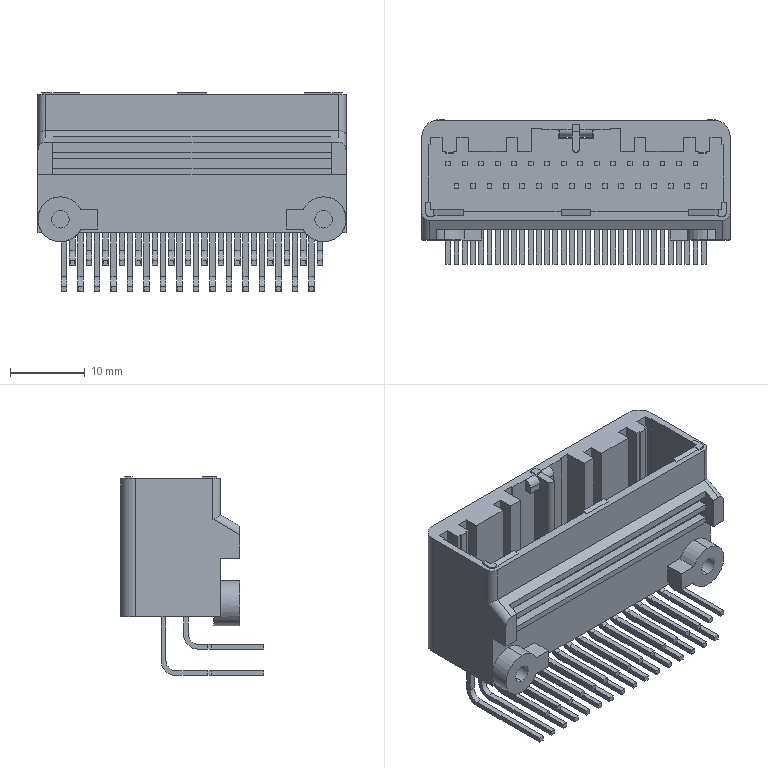Part | SolidWorks | features BaseBody 1 | 1 solid | 733 faces | box 41.1 x 19.2 x 26.52 mm | volume 5328 mm3 | plane 648 | cylinder 85 | commonest cylinder face diameters 2.64 x32 3.92 x32 6 x6 2 x4 2.35 x4 1 x3